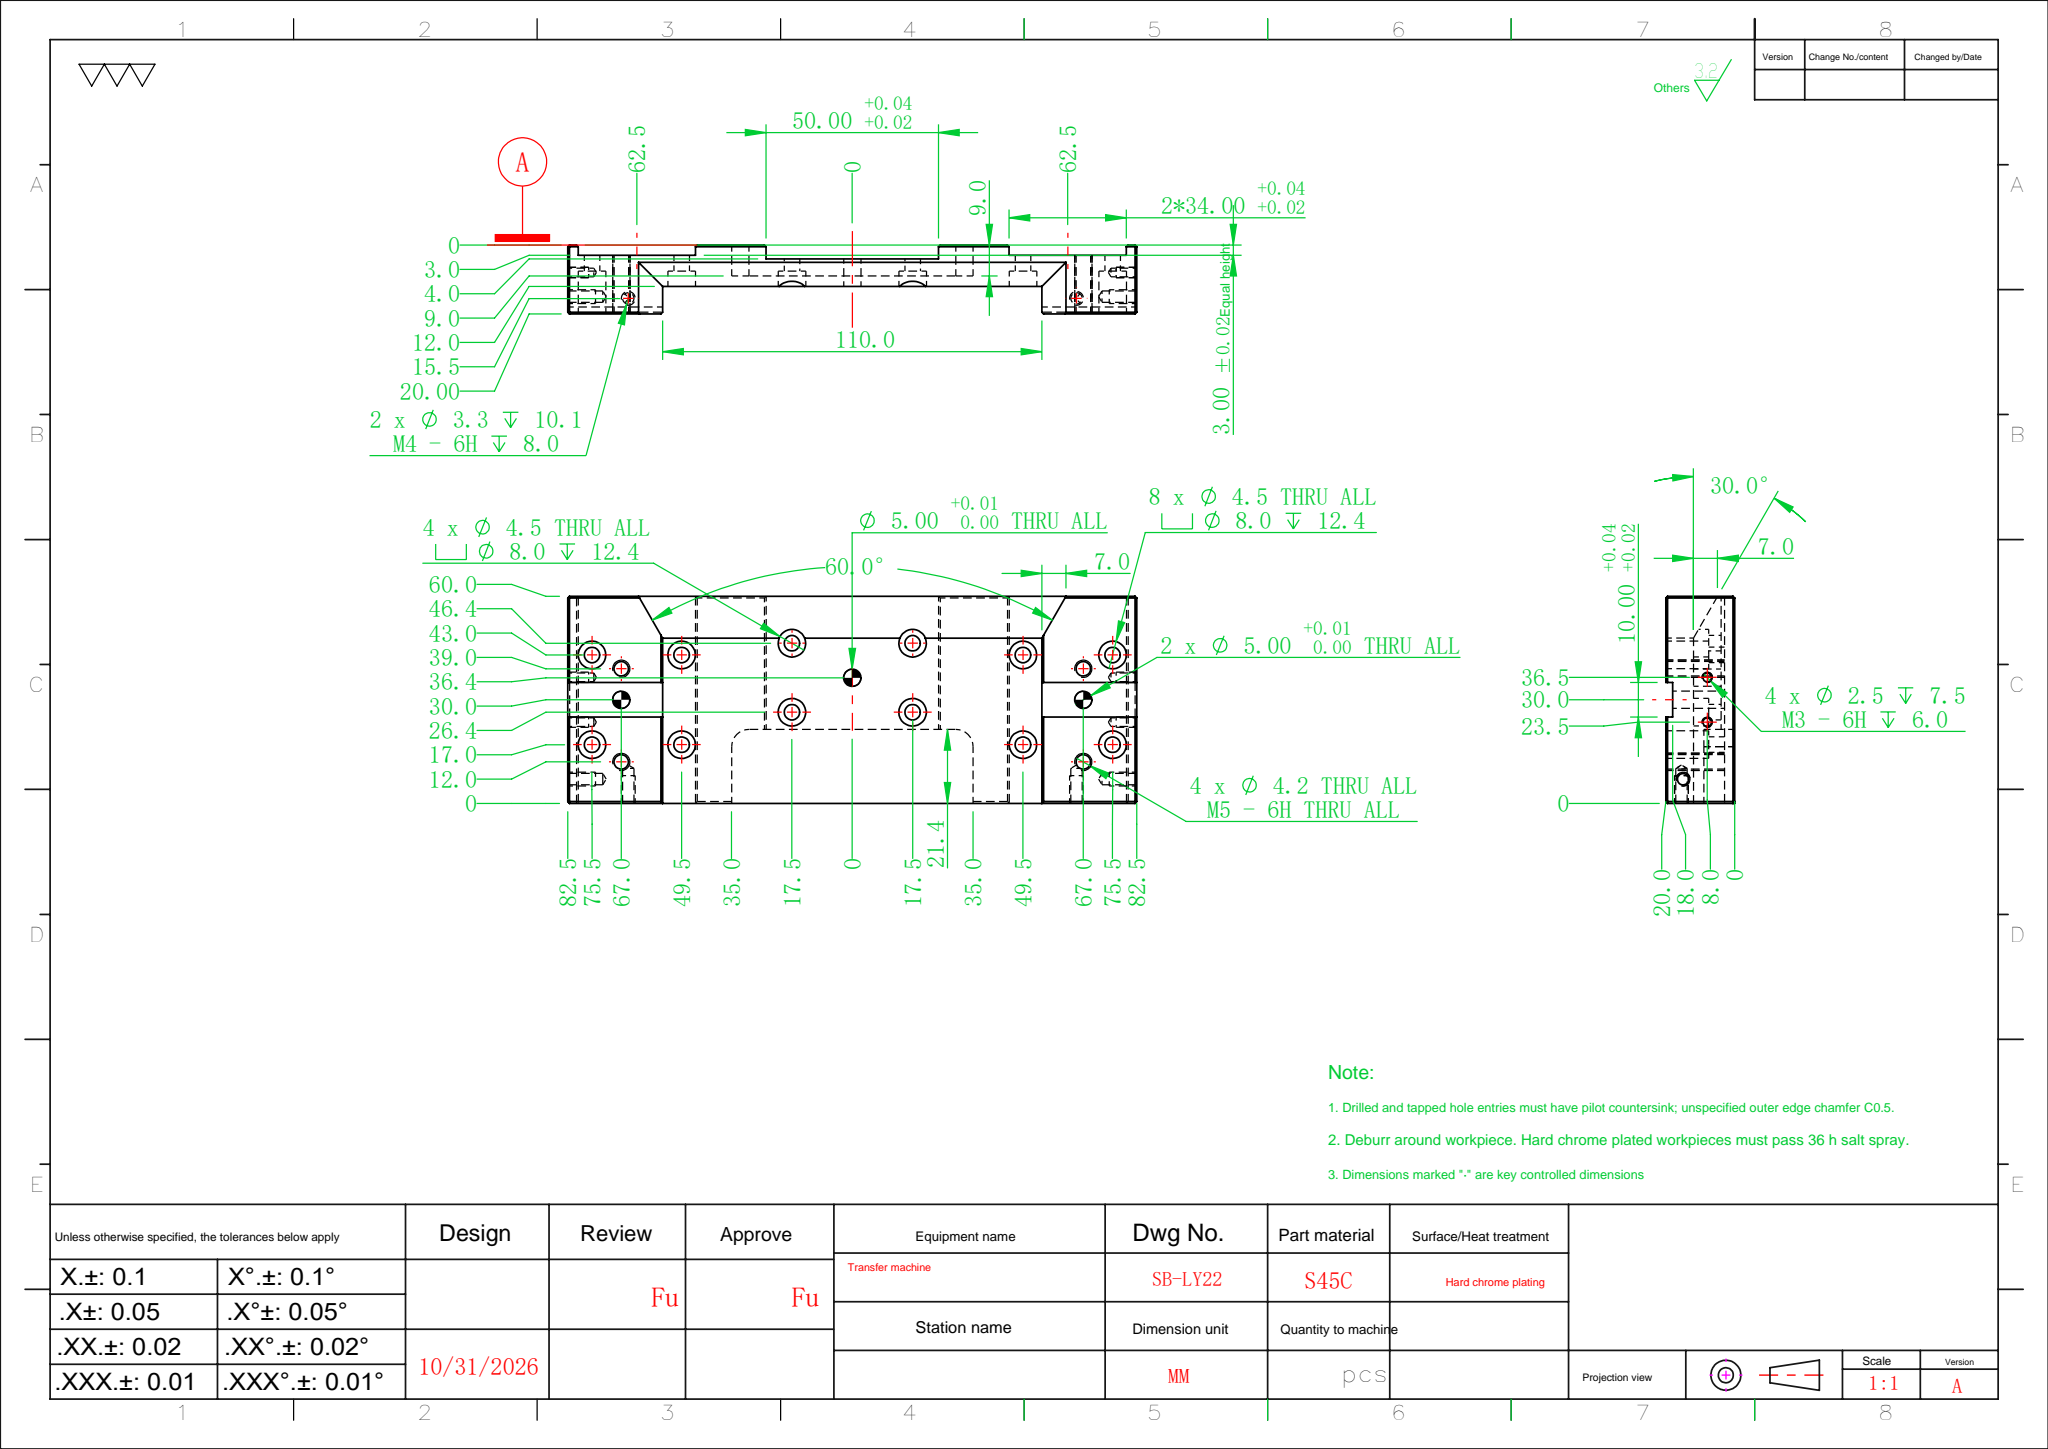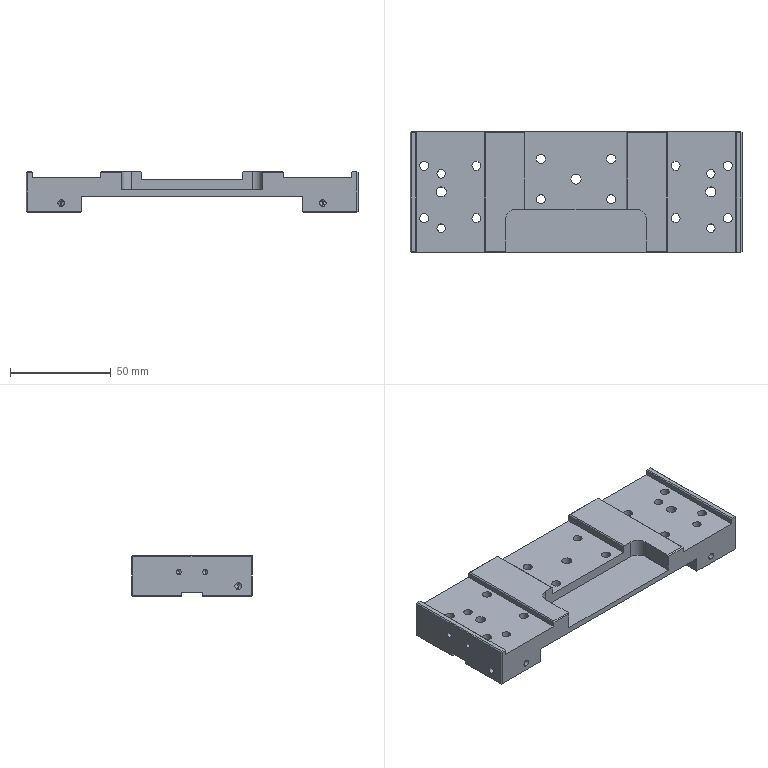Part | SolidWorks | features HoleWzd 8, Cut 4, Chamfer 2, ICE 2, MirrorPattern 2, Extrusion 1, Fillet 1 | 1 solid | 183 faces | box 165 x 60 x 20 mm | volume 97648 mm3 | plane 87 | cylinder 80 | cone 16 | commonest cylinder face diameters 4.5 x24 8 x24 2.5 x8 3.3 x8 4.2 x8 5 x6